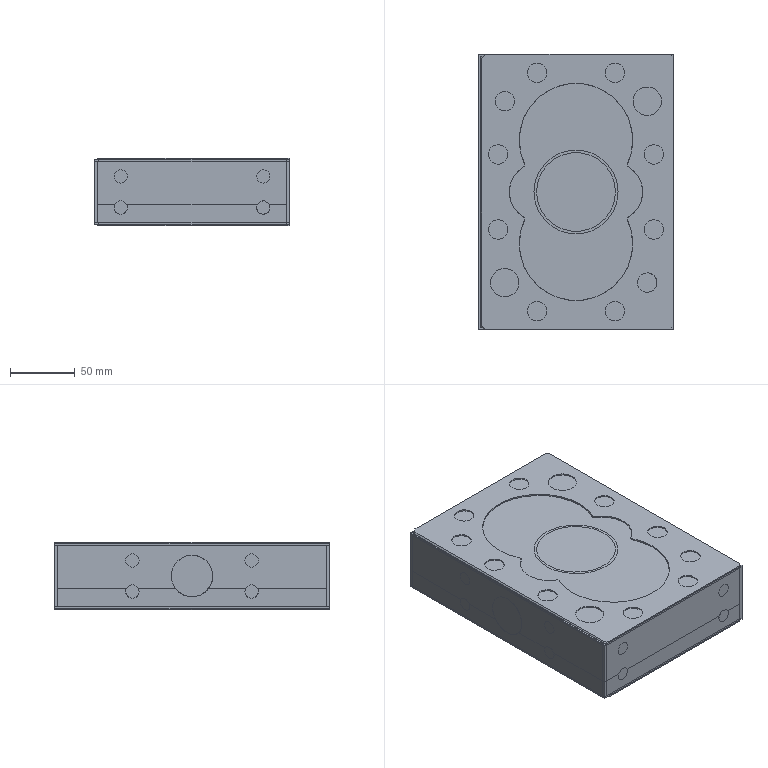NC program | NX | posted with a generic post | part box 150.2 x 212.2 x 52.4 mm
Lines 10238 to 10318 of 152230:
(G81点孔 , TOOL : D6点孔钻_1)
N20468 T01 M6
N20470 /M1
N20472 G54
N20474 G17 G0 G90 X92. Y-30. S1500 M3
N20476 G43 Z100. H1
N20478 G94 G81 G99 Z-1.5 F60. R1.5
N20480 G0 Z100.
N20482 G81 X70. Y-55. Z-1.5 R1.5
N20484 G0 Z100.
N20486 G81 X29. Y-60. Z-1.5 R1.5
N20488 G0 Z100.
N20490 G81 X-29. Z-1.5 R1.5
N20492 G0 Z100.
N20494 G81 X-70. Y-55. Z-1.5 R1.5
N20496 G0 Z100.
N20498 G81 X-92. Y-30. Z-1.5 R1.5
N20500 G0 Z100.
N20502 G81 Y30. Z-1.5 R1.5
N20504 G0 Z100.
N20506 G81 X-70. Y55. Z-1.5 R1.5
N20508 G0 Z100.
N20510 G81 X-29. Y60. Z-1.5 R1.5
N20512 G0 Z100.
N20514 G81 X29. Z-1.5 R1.5
N20516 G0 Z100.
N20518 G81 X70. Y55. Z-1.5 R1.5
N20520 G0 Z100.
N20522 G81 X92. Y30. Z-1.5 R1.5
N20524 G0 Z100.
N20526 G80
N20528 G0 X92. Y30. Z100.
N20530 M5
(G83钻孔 , TOOL : Z8.5钻头)
N20532 T02 M6
N20534 /M1
N20536 G54
N20538 G17 G0 G90 X70. Y55. S800 M3
N20540 G43 Z100. H2
N20542 G94 G83 G99 Z-52. F30. Q52. R1.5
N20544 G0 Z100.
N20546 G83 X92. Y30. Z-52. Q52. R1.5
N20548 G0 Z100.
N20550 G83 Y-30. Z-52. Q52. R1.5
N20552 G0 Z100.
N20554 G83 X29. Y-60. Z-52. Q52. R1.5
N20556 G0 Z100.
N20558 G83 X-29. Z-52. Q52. R1.5
N20560 G0 Z100.
N20562 G83 X-70. Y-55. Z-52. Q52. R1.5
N20564 G0 Z100.
N20566 G83 X-92. Y-30. Z-52. Q52. R1.5
N20568 G0 Z100.
N20570 G83 Y30. Z-52. Q52. R1.5
N20572 G0 Z100.
N20574 G83 X29. Y60. Z-52. Q52. R1.5
N20576 G0 Z100.
N20578 G83 X-29. Z-52. Q52. R1.5
N20580 G0 Z100.
N20582 G80
N20584 G0 X-29. Y60. Z100.
N20586 M5
(G81点孔_1 , TOOL : Z10.3钻头)
N20588 T07 M6
N20590 /M1
N20592 G54
N20594 G17 G0 G90 X-70. Y55. S500 M3
N20596 G43 Z100. H7
N20598 G94 G83 G99 Z-52. F20. Q52. R1.5
N20600 G0 Z100.
N20602 G83 X70. Y-55. Z-52. Q52. R1.5
N20604 G0 Z100.
N20606 G80
N20608 G0 X70. Y-55. Z100.
N20610 M5